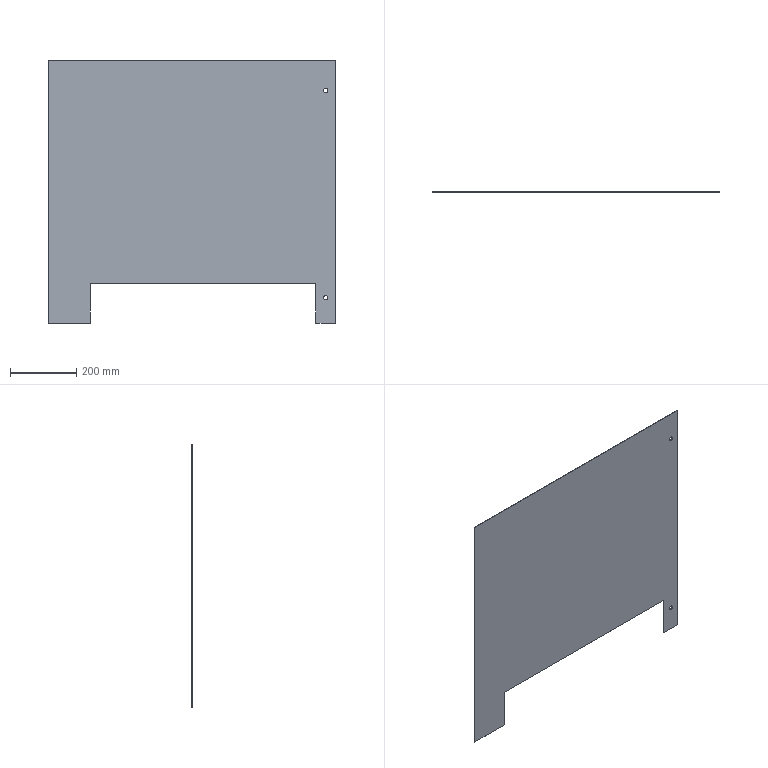Part | STEP file | E3-中转釜花纹Plate 4 | 1 solid | 14 faces | box 867 x 3 x 792 mm | volume 1814396 mm3 | plane 10 | cylinder 4 | commonest cylinder face diameters 13 x4
STEP:
#1=CARTESIAN_POINT('',(0.,0.,0.));
#2=DIRECTION('',(0.,0.,1.));
#3=DIRECTION('',(1.,0.,0.));
#4=AXIS2_PLACEMENT_3D('',#1,#2,#3);
#5=CARTESIAN_POINT('',(837.,0.,-49.5));
#6=VERTEX_POINT('',#5);
#7=CARTESIAN_POINT('',(837.,3.,-49.5));
#8=VERTEX_POINT('',#7);
#9=CARTESIAN_POINT('',(837.,11.,-49.5));
#10=DIRECTION('',(0.,1.,0.));
#11=VECTOR('',#10,1.);
#12=LINE('',#9,#11);
#13=CARTESIAN_POINT('',(837.,11.,-43.));
#14=DIRECTION('',(0.,1.,0.));
#15=DIRECTION('',(0.,0.,-1.));
#16=AXIS2_PLACEMENT_3D('',#13,#14,#15);
#17=CYLINDRICAL_SURFACE('',#16,6.5);
#18=CARTESIAN_POINT('',(6.283,0.));
#19=DIRECTION('',(0.,1.));
#20=VECTOR('',#19,1.);
#21=LINE('',#18,#20);
#22=(GEOMETRIC_REPRESENTATION_CONTEXT(2)PARAMETRIC_REPRESENTATION_CONTEXT()REPRESENTATION_CONTEXT('',''));
#23=DEFINITIONAL_REPRESENTATION('',(#21),#22);
#24=PCURVE('',#17,#23);
#25=CARTESIAN_POINT('',(837.,11.,-43.));
#26=DIRECTION('',(0.,1.,0.));
#27=DIRECTION('',(0.,0.,-1.));
#28=AXIS2_PLACEMENT_3D('',#25,#26,#27);
#29=CYLINDRICAL_SURFACE('',#28,6.5);
#30=CARTESIAN_POINT('',(0.,0.));
#31=DIRECTION('',(0.,1.));
#32=VECTOR('',#31,1.);
#33=LINE('',#30,#32);
#34=(GEOMETRIC_REPRESENTATION_CONTEXT(2)PARAMETRIC_REPRESENTATION_CONTEXT()REPRESENTATION_CONTEXT('',''));
#35=DEFINITIONAL_REPRESENTATION('',(#33),#34);
#36=PCURVE('',#29,#35);
#37=SURFACE_CURVE('',#12,(#24,#36),.PCURVE_S1.);
#38=EDGE_CURVE('',#6,#8,#37,.T.);
#39=ORIENTED_EDGE('',*,*,#38,.T.);
#40=CARTESIAN_POINT('',(837.,3.,-36.5));
#41=VERTEX_POINT('',#40);
#42=CARTESIAN_POINT('',(837.,3.,-43.));
#43=DIRECTION('',(0.,1.,0.));
#44=DIRECTION('',(0.,0.,1.));
#45=AXIS2_PLACEMENT_3D('',#42,#43,#44);
#46=CIRCLE('',#45,6.5);
#47=CARTESIAN_POINT('',(3.142,-8.));
#48=DIRECTION('',(1.,0.));
#49=VECTOR('',#48,1.);
#50=LINE('',#47,#49);
#51=(GEOMETRIC_REPRESENTATION_CONTEXT(2)PARAMETRIC_REPRESENTATION_CONTEXT()REPRESENTATION_CONTEXT('',''));
#52=DEFINITIONAL_REPRESENTATION('',(#50),#51);
#53=PCURVE('',#17,#52);
#54=CARTESIAN_POINT('',(0.,3.,0.));
#55=DIRECTION('',(0.,-1.,0.));
#56=DIRECTION('',(0.,0.,1.));
#57=AXIS2_PLACEMENT_3D('',#54,#55,#56);
#58=PLANE('',#57);
#59=CARTESIAN_POINT('',(-36.5,-837.));
#60=CARTESIAN_POINT('',(-36.5,-848.258));
#61=CARTESIAN_POINT('',(-46.25,-842.629));
#62=CARTESIAN_POINT('',(-56.,-837.));
#63=CARTESIAN_POINT('',(-46.25,-831.371));
#64=CARTESIAN_POINT('',(-36.5,-825.742));
#65=CARTESIAN_POINT('',(-36.5,-837.));
#66=(BOUNDED_CURVE()B_SPLINE_CURVE(2,(#59,#60,#61,#62,#63,#64,#65),.UNSPECIFIED.,.T.,.F.)B_SPLINE_CURVE_WITH_KNOTS((1,2,2,2,2,1),(-2.094,0.,2.094,4.189,6.283,8.378),.UNSPECIFIED.)CURVE()GEOMETRIC_REPRESENTATION_ITEM()RATIONAL_B_SPLINE_CURVE((1.,0.5,1.,0.5,1.,0.5,1.))REPRESENTATION_ITEM(''));
#67=(GEOMETRIC_REPRESENTATION_CONTEXT(2)PARAMETRIC_REPRESENTATION_CONTEXT()REPRESENTATION_CONTEXT('',''));
#68=DEFINITIONAL_REPRESENTATION('',(#66),#67);
#69=PCURVE('',#58,#68);
#70=SURFACE_CURVE('',#46,(#53,#69),.PCURVE_S1.);
#71=EDGE_CURVE('',#41,#8,#70,.T.);
#72=ORIENTED_EDGE('',*,*,#71,.F.);
#73=CARTESIAN_POINT('',(837.,0.,-36.5));
#74=VERTEX_POINT('',#73);
#75=CARTESIAN_POINT('',(837.,11.,-36.5));
#76=DIRECTION('',(0.,1.,0.));
#77=VECTOR('',#76,1.);
#78=LINE('',#75,#77);
#79=CARTESIAN_POINT('',(3.142,0.));
#80=DIRECTION('',(0.,1.));
#81=VECTOR('',#80,1.);
#82=LINE('',#79,#81);
#83=(GEOMETRIC_REPRESENTATION_CONTEXT(2)PARAMETRIC_REPRESENTATION_CONTEXT()REPRESENTATION_CONTEXT('',''));
#84=DEFINITIONAL_REPRESENTATION('',(#82),#83);
#85=PCURVE('',#17,#84);
#86=CARTESIAN_POINT('',(3.142,0.));
#87=DIRECTION('',(0.,1.));
#88=VECTOR('',#87,1.);
#89=LINE('',#86,#88);
#90=(GEOMETRIC_REPRESENTATION_CONTEXT(2)PARAMETRIC_REPRESENTATION_CONTEXT()REPRESENTATION_CONTEXT('',''));
#91=DEFINITIONAL_REPRESENTATION('',(#89),#90);
#92=PCURVE('',#29,#91);
#93=SURFACE_CURVE('',#78,(#85,#92),.PCURVE_S1.);
#94=EDGE_CURVE('',#74,#41,#93,.T.);
#95=ORIENTED_EDGE('',*,*,#94,.F.);
#96=CARTESIAN_POINT('',(837.,0.,-43.));
#97=DIRECTION('',(0.,1.,0.));
#98=DIRECTION('',(0.,0.,1.));
#99=AXIS2_PLACEMENT_3D('',#96,#97,#98);
#100=CIRCLE('',#99,6.5);
#101=CARTESIAN_POINT('',(3.142,-11.));
#102=DIRECTION('',(1.,0.));
#103=VECTOR('',#102,1.);
#104=LINE('',#101,#103);
#105=(GEOMETRIC_REPRESENTATION_CONTEXT(2)PARAMETRIC_REPRESENTATION_CONTEXT()REPRESENTATION_CONTEXT('',''));
#106=DEFINITIONAL_REPRESENTATION('',(#104),#105);
#107=PCURVE('',#17,#106);
#108=CARTESIAN_POINT('',(0.,0.,0.));
#109=DIRECTION('',(0.,-1.,0.));
#110=DIRECTION('',(0.,0.,1.));
#111=AXIS2_PLACEMENT_3D('',#108,#109,#110);
#112=PLANE('',#111);
#113=CARTESIAN_POINT('',(-36.5,-837.));
#114=CARTESIAN_POINT('',(-36.5,-848.258));
#115=CARTESIAN_POINT('',(-46.25,-842.629));
#116=CARTESIAN_POINT('',(-56.,-837.));
#117=CARTESIAN_POINT('',(-46.25,-831.371));
#118=CARTESIAN_POINT('',(-36.5,-825.742));
#119=CARTESIAN_POINT('',(-36.5,-837.));
#120=(BOUNDED_CURVE()B_SPLINE_CURVE(2,(#113,#114,#115,#116,#117,#118,#119),.UNSPECIFIED.,.T.,.F.)B_SPLINE_CURVE_WITH_KNOTS((1,2,2,2,2,1),(-2.094,0.,2.094,4.189,6.283,8.378),.UNSPECIFIED.)CURVE()GEOMETRIC_REPRESENTATION_ITEM()RATIONAL_B_SPLINE_CURVE((1.,0.5,1.,0.5,1.,0.5,1.))REPRESENTATION_ITEM(''));
#121=(GEOMETRIC_REPRESENTATION_CONTEXT(2)PARAMETRIC_REPRESENTATION_CONTEXT()REPRESENTATION_CONTEXT('',''));
#122=DEFINITIONAL_REPRESENTATION('',(#120),#121);
#123=PCURVE('',#112,#122);
#124=SURFACE_CURVE('',#100,(#107,#123),.PCURVE_S1.);
#125=EDGE_CURVE('',#74,#6,#124,.T.);
#126=ORIENTED_EDGE('',*,*,#125,.T.);
#127=EDGE_LOOP('',(#39,#72,#95,#126));
#128=FACE_BOUND('',#127,.F.);
#129=ADVANCED_FACE('',(#128),#17,.F.);
#130=CARTESIAN_POINT('',(837.,0.,575.5));
#131=VERTEX_POINT('',#130);
#132=CARTESIAN_POINT('',(837.,3.,575.5));
#133=VERTEX_POINT('',#132);
#134=CARTESIAN_POINT('',(837.,11.,575.5));
#135=DIRECTION('',(0.,1.,0.));
#136=VECTOR('',#135,1.);
#137=LINE('',#134,#136);
#138=CARTESIAN_POINT('',(837.,11.,582.));
#139=DIRECTION('',(0.,1.,0.));
#140=DIRECTION('',(0.,0.,-1.));
#141=AXIS2_PLACEMENT_3D('',#138,#139,#140);
#142=CYLINDRICAL_SURFACE('',#141,6.5);
#143=CARTESIAN_POINT('',(6.283,0.));
#144=DIRECTION('',(0.,1.));
#145=VECTOR('',#144,1.);
#146=LINE('',#143,#145);
#147=(GEOMETRIC_REPRESENTATION_CONTEXT(2)PARAMETRIC_REPRESENTATION_CONTEXT()REPRESENTATION_CONTEXT('',''));
#148=DEFINITIONAL_REPRESENTATION('',(#146),#147);
#149=PCURVE('',#142,#148);
#150=CARTESIAN_POINT('',(837.,11.,582.));
#151=DIRECTION('',(0.,1.,0.));
#152=DIRECTION('',(0.,0.,-1.));
#153=AXIS2_PLACEMENT_3D('',#150,#151,#152);
#154=CYLINDRICAL_SURFACE('',#153,6.5);
#155=CARTESIAN_POINT('',(0.,0.));
#156=DIRECTION('',(0.,1.));
#157=VECTOR('',#156,1.);
#158=LINE('',#155,#157);
#159=(GEOMETRIC_REPRESENTATION_CONTEXT(2)PARAMETRIC_REPRESENTATION_CONTEXT()REPRESENTATION_CONTEXT('',''));
#160=DEFINITIONAL_REPRESENTATION('',(#158),#159);
#161=PCURVE('',#154,#160);
#162=SURFACE_CURVE('',#137,(#149,#161),.PCURVE_S1.);
#163=EDGE_CURVE('',#131,#133,#162,.T.);
#164=ORIENTED_EDGE('',*,*,#163,.T.);
#165=CARTESIAN_POINT('',(837.,3.,588.5));
#166=VERTEX_POINT('',#165);
#167=CARTESIAN_POINT('',(837.,3.,582.));
#168=DIRECTION('',(0.,1.,0.));
#169=DIRECTION('',(0.,0.,1.));
#170=AXIS2_PLACEMENT_3D('',#167,#168,#169);
#171=CIRCLE('',#170,6.5);
#172=CARTESIAN_POINT('',(3.142,-8.));
#173=DIRECTION('',(1.,0.));
#174=VECTOR('',#173,1.);
#175=LINE('',#172,#174);
#176=(GEOMETRIC_REPRESENTATION_CONTEXT(2)PARAMETRIC_REPRESENTATION_CONTEXT()REPRESENTATION_CONTEXT('',''));
#177=DEFINITIONAL_REPRESENTATION('',(#175),#176);
#178=PCURVE('',#142,#177);
#179=CARTESIAN_POINT('',(588.5,-837.));
#180=CARTESIAN_POINT('',(588.5,-848.258));
#181=CARTESIAN_POINT('',(578.75,-842.629));
#182=CARTESIAN_POINT('',(569.,-837.));
#183=CARTESIAN_POINT('',(578.75,-831.371));
#184=CARTESIAN_POINT('',(588.5,-825.742));
#185=CARTESIAN_POINT('',(588.5,-837.));
#186=(BOUNDED_CURVE()B_SPLINE_CURVE(2,(#179,#180,#181,#182,#183,#184,#185),.UNSPECIFIED.,.T.,.F.)B_SPLINE_CURVE_WITH_KNOTS((1,2,2,2,2,1),(-2.094,0.,2.094,4.189,6.283,8.378),.UNSPECIFIED.)CURVE()GEOMETRIC_REPRESENTATION_ITEM()RATIONAL_B_SPLINE_CURVE((1.,0.5,1.,0.5,1.,0.5,1.))REPRESENTATION_ITEM(''));
#187=(GEOMETRIC_REPRESENTATION_CONTEXT(2)PARAMETRIC_REPRESENTATION_CONTEXT()REPRESENTATION_CONTEXT('',''));
#188=DEFINITIONAL_REPRESENTATION('',(#186),#187);
#189=PCURVE('',#58,#188);
#190=SURFACE_CURVE('',#171,(#178,#189),.PCURVE_S1.);
#191=EDGE_CURVE('',#166,#133,#190,.T.);
#192=ORIENTED_EDGE('',*,*,#191,.F.);
#193=CARTESIAN_POINT('',(837.,0.,588.5));
#194=VERTEX_POINT('',#193);
#195=CARTESIAN_POINT('',(837.,11.,588.5));
#196=DIRECTION('',(0.,1.,0.));
#197=VECTOR('',#196,1.);
#198=LINE('',#195,#197);
#199=CARTESIAN_POINT('',(3.142,0.));
#200=DIRECTION('',(0.,1.));
#201=VECTOR('',#200,1.);
#202=LINE('',#199,#201);
#203=(GEOMETRIC_REPRESENTATION_CONTEXT(2)PARAMETRIC_REPRESENTATION_CONTEXT()REPRESENTATION_CONTEXT('',''));
#204=DEFINITIONAL_REPRESENTATION('',(#202),#203);
#205=PCURVE('',#142,#204);
#206=CARTESIAN_POINT('',(3.142,0.));
#207=DIRECTION('',(0.,1.));
#208=VECTOR('',#207,1.);
#209=LINE('',#206,#208);
#210=(GEOMETRIC_REPRESENTATION_CONTEXT(2)PARAMETRIC_REPRESENTATION_CONTEXT()REPRESENTATION_CONTEXT('',''));
#211=DEFINITIONAL_REPRESENTATION('',(#209),#210);
#212=PCURVE('',#154,#211);
#213=SURFACE_CURVE('',#198,(#205,#212),.PCURVE_S1.);
#214=EDGE_CURVE('',#194,#166,#213,.T.);
#215=ORIENTED_EDGE('',*,*,#214,.F.);
#216=CARTESIAN_POINT('',(837.,0.,582.));
#217=DIRECTION('',(0.,1.,0.));
#218=DIRECTION('',(0.,0.,1.));
#219=AXIS2_PLACEMENT_3D('',#216,#217,#218);
#220=CIRCLE('',#219,6.5);
#221=CARTESIAN_POINT('',(3.142,-11.));
#222=DIRECTION('',(1.,0.));
#223=VECTOR('',#222,1.);
#224=LINE('',#221,#223);
#225=(GEOMETRIC_REPRESENTATION_CONTEXT(2)PARAMETRIC_REPRESENTATION_CONTEXT()REPRESENTATION_CONTEXT('',''));
#226=DEFINITIONAL_REPRESENTATION('',(#224),#225);
#227=PCURVE('',#142,#226);
#228=CARTESIAN_POINT('',(588.5,-837.));
#229=CARTESIAN_POINT('',(588.5,-848.258));
#230=CARTESIAN_POINT('',(578.75,-842.629));
#231=CARTESIAN_POINT('',(569.,-837.));
#232=CARTESIAN_POINT('',(578.75,-831.371));
#233=CARTESIAN_POINT('',(588.5,-825.742));
#234=CARTESIAN_POINT('',(588.5,-837.));
#235=(BOUNDED_CURVE()B_SPLINE_CURVE(2,(#228,#229,#230,#231,#232,#233,#234),.UNSPECIFIED.,.T.,.F.)B_SPLINE_CURVE_WITH_KNOTS((1,2,2,2,2,1),(-2.094,0.,2.094,4.189,6.283,8.378),.UNSPECIFIED.)CURVE()GEOMETRIC_REPRESENTATION_ITEM()RATIONAL_B_SPLINE_CURVE((1.,0.5,1.,0.5,1.,0.5,1.))REPRESENTATION_ITEM(''));
#236=(GEOMETRIC_REPRESENTATION_CONTEXT(2)PARAMETRIC_REPRESENTATION_CONTEXT()REPRESENTATION_CONTEXT('',''));
#237=DEFINITIONAL_REPRESENTATION('',(#235),#236);
#238=PCURVE('',#112,#237);
#239=SURFACE_CURVE('',#220,(#227,#238),.PCURVE_S1.);
#240=EDGE_CURVE('',#194,#131,#239,.T.);
#241=ORIENTED_EDGE('',*,*,#240,.T.);
#242=EDGE_LOOP('',(#164,#192,#215,#241));
#243=FACE_BOUND('',#242,.F.);
#244=ADVANCED_FACE('',(#243),#142,.F.);
#245=CARTESIAN_POINT('',(127.,0.,0.));
#246=VERTEX_POINT('',#245);
#247=CARTESIAN_POINT('',(807.,0.,0.));
#248=VERTEX_POINT('',#247);
#249=CARTESIAN_POINT('',(0.,0.,0.));
#250=DIRECTION('',(1.,0.,0.));
#251=VECTOR('',#250,1.);
#252=LINE('',#249,#251);
#253=CARTESIAN_POINT('',(0.,3.,0.));
#254=DIRECTION('',(0.,0.,1.));
#255=DIRECTION('',(-1.,0.,0.));
#256=AXIS2_PLACEMENT_3D('',#253,#254,#255);
#257=PLANE('',#256);
#258=CARTESIAN_POINT('',(0.,3.));
#259=DIRECTION('',(-1.,0.));
#260=VECTOR('',#259,1.);
#261=LINE('',#258,#260);
#262=(GEOMETRIC_REPRESENTATION_CONTEXT(2)PARAMETRIC_REPRESENTATION_CONTEXT()REPRESENTATION_CONTEXT('',''));
#263=DEFINITIONAL_REPRESENTATION('',(#261),#262);
#264=PCURVE('',#257,#263);
#265=CARTESIAN_POINT('',(0.,0.));
#266=DIRECTION('',(0.,-1.));
#267=VECTOR('',#266,1.);
#268=LINE('',#265,#267);
#269=(GEOMETRIC_REPRESENTATION_CONTEXT(2)PARAMETRIC_REPRESENTATION_CONTEXT()REPRESENTATION_CONTEXT('',''));
#270=DEFINITIONAL_REPRESENTATION('',(#268),#269);
#271=PCURVE('',#112,#270);
#272=SURFACE_CURVE('',#252,(#264,#271),.PCURVE_S1.);
#273=EDGE_CURVE('',#246,#248,#272,.T.);
#274=ORIENTED_EDGE('',*,*,#273,.F.);
#275=CARTESIAN_POINT('',(127.,3.,0.));
#276=VERTEX_POINT('',#275);
#277=CARTESIAN_POINT('',(127.,0.,0.));
#278=DIRECTION('',(0.,1.,0.));
#279=VECTOR('',#278,1.);
#280=LINE('',#277,#279);
#281=CARTESIAN_POINT('',(-127.,3.));
#282=DIRECTION('',(0.,-1.));
#283=VECTOR('',#282,1.);
#284=LINE('',#281,#283);
#285=(GEOMETRIC_REPRESENTATION_CONTEXT(2)PARAMETRIC_REPRESENTATION_CONTEXT()REPRESENTATION_CONTEXT('',''));
#286=DEFINITIONAL_REPRESENTATION('',(#284),#285);
#287=PCURVE('',#257,#286);
#288=CARTESIAN_POINT('',(127.,0.,0.));
#289=DIRECTION('',(1.,0.,0.));
#290=DIRECTION('',(0.,0.,1.));
#291=AXIS2_PLACEMENT_3D('',#288,#289,#290);
#292=PLANE('',#291);
#293=CARTESIAN_POINT('',(0.,0.));
#294=DIRECTION('',(0.,-1.));
#295=VECTOR('',#294,1.);
#296=LINE('',#293,#295);
#297=(GEOMETRIC_REPRESENTATION_CONTEXT(2)PARAMETRIC_REPRESENTATION_CONTEXT()REPRESENTATION_CONTEXT('',''));
#298=DEFINITIONAL_REPRESENTATION('',(#296),#297);
#299=PCURVE('',#292,#298);
#300=SURFACE_CURVE('',#280,(#287,#299),.PCURVE_S1.);
#301=EDGE_CURVE('',#246,#276,#300,.T.);
#302=ORIENTED_EDGE('',*,*,#301,.T.);
#303=CARTESIAN_POINT('',(807.,3.,0.));
#304=VERTEX_POINT('',#303);
#305=CARTESIAN_POINT('',(0.,3.,0.));
#306=DIRECTION('',(1.,0.,0.));
#307=VECTOR('',#306,1.);
#308=LINE('',#305,#307);
#309=CARTESIAN_POINT('',(0.,0.));
#310=DIRECTION('',(-1.,0.));
#311=VECTOR('',#310,1.);
#312=LINE('',#309,#311);
#313=(GEOMETRIC_REPRESENTATION_CONTEXT(2)PARAMETRIC_REPRESENTATION_CONTEXT()REPRESENTATION_CONTEXT('',''));
#314=DEFINITIONAL_REPRESENTATION('',(#312),#313);
#315=PCURVE('',#257,#314);
#316=CARTESIAN_POINT('',(0.,0.));
#317=DIRECTION('',(0.,-1.));
#318=VECTOR('',#317,1.);
#319=LINE('',#316,#318);
#320=(GEOMETRIC_REPRESENTATION_CONTEXT(2)PARAMETRIC_REPRESENTATION_CONTEXT()REPRESENTATION_CONTEXT('',''));
#321=DEFINITIONAL_REPRESENTATION('',(#319),#320);
#322=PCURVE('',#58,#321);
#323=SURFACE_CURVE('',#308,(#315,#322),.PCURVE_S1.);
#324=EDGE_CURVE('',#276,#304,#323,.T.);
#325=ORIENTED_EDGE('',*,*,#324,.T.);
#326=CARTESIAN_POINT('',(807.,0.,0.));
#327=DIRECTION('',(0.,1.,0.));
#328=VECTOR('',#327,1.);
#329=LINE('',#326,#328);
#330=CARTESIAN_POINT('',(-807.,3.));
#331=DIRECTION('',(0.,-1.));
#332=VECTOR('',#331,1.);
#333=LINE('',#330,#332);
#334=(GEOMETRIC_REPRESENTATION_CONTEXT(2)PARAMETRIC_REPRESENTATION_CONTEXT()REPRESENTATION_CONTEXT('',''));
#335=DEFINITIONAL_REPRESENTATION('',(#333),#334);
#336=PCURVE('',#257,#335);
#337=CARTESIAN_POINT('',(807.,0.,0.));
#338=DIRECTION('',(-1.,0.,0.));
#339=DIRECTION('',(0.,0.,-1.));
#340=AXIS2_PLACEMENT_3D('',#337,#338,#339);
#341=PLANE('',#340);
#342=CARTESIAN_POINT('',(0.,0.));
#343=DIRECTION('',(0.,-1.));
#344=VECTOR('',#343,1.);
#345=LINE('',#342,#344);
#346=(GEOMETRIC_REPRESENTATION_CONTEXT(2)PARAMETRIC_REPRESENTATION_CONTEXT()REPRESENTATION_CONTEXT('',''));
#347=DEFINITIONAL_REPRESENTATION('',(#345),#346);
#348=PCURVE('',#341,#347);
#349=SURFACE_CURVE('',#329,(#336,#348),.PCURVE_S1.);
#350=EDGE_CURVE('',#248,#304,#349,.T.);
#351=ORIENTED_EDGE('',*,*,#350,.F.);
#352=EDGE_LOOP('',(#274,#302,#325,#351));
#353=FACE_BOUND('',#352,.T.);
#354=ADVANCED_FACE('',(#353),#257,.F.);
#355=CARTESIAN_POINT('',(0.,0.,672.));
#356=VERTEX_POINT('',#355);
#357=CARTESIAN_POINT('',(0.,0.,-120.));
#358=VERTEX_POINT('',#357);
#359=CARTESIAN_POINT('',(0.,0.,0.));
#360=DIRECTION('',(0.,0.,-1.));
#361=VECTOR('',#360,1.);
#362=LINE('',#359,#361);
#363=CARTESIAN_POINT('',(0.,3.,0.));
#364=DIRECTION('',(1.,0.,0.));
#365=DIRECTION('',(0.,0.,1.));
#366=AXIS2_PLACEMENT_3D('',#363,#364,#365);
#367=PLANE('',#366);
#368=CARTESIAN_POINT('',(0.,3.));
#369=DIRECTION('',(-1.,0.));
#370=VECTOR('',#369,1.);
#371=LINE('',#368,#370);
#372=(GEOMETRIC_REPRESENTATION_CONTEXT(2)PARAMETRIC_REPRESENTATION_CONTEXT()REPRESENTATION_CONTEXT('',''));
#373=DEFINITIONAL_REPRESENTATION('',(#371),#372);
#374=PCURVE('',#367,#373);
#375=CARTESIAN_POINT('',(0.,0.));
#376=DIRECTION('',(-1.,0.));
#377=VECTOR('',#376,1.);
#378=LINE('',#375,#377);
#379=(GEOMETRIC_REPRESENTATION_CONTEXT(2)PARAMETRIC_REPRESENTATION_CONTEXT()REPRESENTATION_CONTEXT('',''));
#380=DEFINITIONAL_REPRESENTATION('',(#378),#379);
#381=PCURVE('',#112,#380);
#382=SURFACE_CURVE('',#362,(#374,#381),.PCURVE_S1.);
#383=EDGE_CURVE('',#356,#358,#382,.T.);
#384=ORIENTED_EDGE('',*,*,#383,.F.);
#385=CARTESIAN_POINT('',(0.,3.,672.));
#386=VERTEX_POINT('',#385);
#387=CARTESIAN_POINT('',(0.,3.,672.));
#388=DIRECTION('',(0.,-1.,0.));
#389=VECTOR('',#388,1.);
#390=LINE('',#387,#389);
#391=CARTESIAN_POINT('',(672.,0.));
#392=DIRECTION('',(0.,1.));
#393=VECTOR('',#392,1.);
#394=LINE('',#391,#393);
#395=(GEOMETRIC_REPRESENTATION_CONTEXT(2)PARAMETRIC_REPRESENTATION_CONTEXT()REPRESENTATION_CONTEXT('',''));
#396=DEFINITIONAL_REPRESENTATION('',(#394),#395);
#397=PCURVE('',#367,#396);
#398=CARTESIAN_POINT('',(0.,3.,672.));
#399=DIRECTION('',(0.,0.,-1.));
#400=DIRECTION('',(1.,0.,0.));
#401=AXIS2_PLACEMENT_3D('',#398,#399,#400);
#402=PLANE('',#401);
#403=CARTESIAN_POINT('',(0.,0.));
#404=DIRECTION('',(0.,1.));
#405=VECTOR('',#404,1.);
#406=LINE('',#403,#405);
#407=(GEOMETRIC_REPRESENTATION_CONTEXT(2)PARAMETRIC_REPRESENTATION_CONTEXT()REPRESENTATION_CONTEXT('',''));
#408=DEFINITIONAL_REPRESENTATION('',(#406),#407);
#409=PCURVE('',#402,#408);
#410=SURFACE_CURVE('',#390,(#397,#409),.PCURVE_S1.);
#411=EDGE_CURVE('',#386,#356,#410,.T.);
#412=ORIENTED_EDGE('',*,*,#411,.F.);
#413=CARTESIAN_POINT('',(0.,3.,-120.));
#414=VERTEX_POINT('',#413);
#415=CARTESIAN_POINT('',(0.,3.,0.));
#416=DIRECTION('',(0.,0.,-1.));
#417=VECTOR('',#416,1.);
#418=LINE('',#415,#417);
#419=CARTESIAN_POINT('',(0.,0.));
#420=DIRECTION('',(-1.,0.));
#421=VECTOR('',#420,1.);
#422=LINE('',#419,#421);
#423=(GEOMETRIC_REPRESENTATION_CONTEXT(2)PARAMETRIC_REPRESENTATION_CONTEXT()REPRESENTATION_CONTEXT('',''));
#424=DEFINITIONAL_REPRESENTATION('',(#422),#423);
#425=PCURVE('',#367,#424);
#426=CARTESIAN_POINT('',(0.,0.));
#427=DIRECTION('',(-1.,0.));
#428=VECTOR('',#427,1.);
#429=LINE('',#426,#428);
#430=(GEOMETRIC_REPRESENTATION_CONTEXT(2)PARAMETRIC_REPRESENTATION_CONTEXT()REPRESENTATION_CONTEXT('',''));
#431=DEFINITIONAL_REPRESENTATION('',(#429),#430);
#432=PCURVE('',#58,#431);
#433=SURFACE_CURVE('',#418,(#425,#432),.PCURVE_S1.);
#434=EDGE_CURVE('',#386,#414,#433,.T.);
#435=ORIENTED_EDGE('',*,*,#434,.T.);
#436=CARTESIAN_POINT('',(0.,0.,-120.));
#437=DIRECTION('',(0.,1.,0.));
#438=VECTOR('',#437,1.);
#439=LINE('',#436,#438);
#440=CARTESIAN_POINT('',(-120.,3.));
#441=DIRECTION('',(0.,-1.));
#442=VECTOR('',#441,1.);
#443=LINE('',#440,#442);
#444=(GEOMETRIC_REPRESENTATION_CONTEXT(2)PARAMETRIC_REPRESENTATION_CONTEXT()REPRESENTATION_CONTEXT('',''));
#445=DEFINITIONAL_REPRESENTATION('',(#443),#444);
#446=PCURVE('',#367,#445);
#447=CARTESIAN_POINT('',(0.,0.,-120.));
#448=DIRECTION('',(0.,0.,-1.));
#449=DIRECTION('',(1.,0.,0.));
#450=AXIS2_PLACEMENT_3D('',#447,#448,#449);
#451=PLANE('',#450);
#452=CARTESIAN_POINT('',(0.,0.));
#453=DIRECTION('',(0.,-1.));
#454=VECTOR('',#453,1.);
#455=LINE('',#452,#454);
#456=(GEOMETRIC_REPRESENTATION_CONTEXT(2)PARAMETRIC_REPRESENTATION_CONTEXT()REPRESENTATION_CONTEXT('',''));
#457=DEFINITIONAL_REPRESENTATION('',(#455),#456);
#458=PCURVE('',#451,#457);
#459=SURFACE_CURVE('',#439,(#446,#458),.PCURVE_S1.);
#460=EDGE_CURVE('',#358,#414,#459,.T.);
#461=ORIENTED_EDGE('',*,*,#460,.F.);
#462=EDGE_LOOP('',(#384,#412,#435,#461));
#463=FACE_BOUND('',#462,.T.);
#464=ADVANCED_FACE('',(#463),#367,.F.);
#465=CARTESIAN_POINT('',(867.,0.,-120.));
#466=VERTEX_POINT('',#465);
#467=CARTESIAN_POINT('',(867.,0.,672.));
#468=VERTEX_POINT('',#467);
#469=CARTESIAN_POINT('',(867.,0.,0.));
#470=DIRECTION('',(0.,0.,1.));
#471=VECTOR('',#470,1.);
#472=LINE('',#469,#471);
#473=CARTESIAN_POINT('',(867.,3.,0.));
#474=DIRECTION('',(-1.,0.,0.));
#475=DIRECTION('',(0.,0.,-1.));
#476=AXIS2_PLACEMENT_3D('',#473,#474,#475);
#477=PLANE('',#476);
#478=CARTESIAN_POINT('',(0.,3.));
#479=DIRECTION('',(-1.,0.));
#480=VECTOR('',#479,1.);
#481=LINE('',#478,#480);
#482=(GEOMETRIC_REPRESENTATION_CONTEXT(2)PARAMETRIC_REPRESENTATION_CONTEXT()REPRESENTATION_CONTEXT('',''));
#483=DEFINITIONAL_REPRESENTATION('',(#481),#482);
#484=PCURVE('',#477,#483);
#485=CARTESIAN_POINT('',(0.,-867.));
#486=DIRECTION('',(1.,0.));
#487=VECTOR('',#486,1.);
#488=LINE('',#485,#487);
#489=(GEOMETRIC_REPRESENTATION_CONTEXT(2)PARAMETRIC_REPRESENTATION_CONTEXT()REPRESENTATION_CONTEXT('',''));
#490=DEFINITIONAL_REPRESENTATION('',(#488),#489);
#491=PCURVE('',#112,#490);
#492=SURFACE_CURVE('',#472,(#484,#491),.PCURVE_S1.);
#493=EDGE_CURVE('',#466,#468,#492,.T.);
#494=ORIENTED_EDGE('',*,*,#493,.F.);
#495=CARTESIAN_POINT('',(867.,3.,-120.));
#496=VERTEX_POINT('',#495);
#497=CARTESIAN_POINT('',(867.,0.,-120.));
#498=DIRECTION('',(0.,1.,0.));
#499=VECTOR('',#498,1.);
#500=LINE('',#497,#499);
#501=CARTESIAN_POINT('',(120.,3.));
#502=DIRECTION('',(0.,-1.));
#503=VECTOR('',#502,1.);
#504=LINE('',#501,#503);
#505=(GEOMETRIC_REPRESENTATION_CONTEXT(2)PARAMETRIC_REPRESENTATION_CONTEXT()REPRESENTATION_CONTEXT('',''));
#506=DEFINITIONAL_REPRESENTATION('',(#504),#505);
#507=PCURVE('',#477,#506);
#508=CARTESIAN_POINT('',(867.,0.,-120.));
#509=DIRECTION('',(0.,0.,-1.));
#510=DIRECTION('',(1.,0.,0.));
#511=AXIS2_PLACEMENT_3D('',#508,#509,#510);
#512=PLANE('',#511);
#513=CARTESIAN_POINT('',(0.,0.));
#514=DIRECTION('',(0.,-1.));
#515=VECTOR('',#514,1.);
#516=LINE('',#513,#515);
#517=(GEOMETRIC_REPRESENTATION_CONTEXT(2)PARAMETRIC_REPRESENTATION_CONTEXT()REPRESENTATION_CONTEXT('',''));
#518=DEFINITIONAL_REPRESENTATION('',(#516),#517);
#519=PCURVE('',#512,#518);
#520=SURFACE_CURVE('',#500,(#507,#519),.PCURVE_S1.);
#521=EDGE_CURVE('',#466,#496,#520,.T.);
#522=ORIENTED_EDGE('',*,*,#521,.T.);
#523=CARTESIAN_POINT('',(867.,3.,672.));
#524=VERTEX_POINT('',#523);
#525=CARTESIAN_POINT('',(867.,3.,0.));
#526=DIRECTION('',(0.,0.,1.));
#527=VECTOR('',#526,1.);
#528=LINE('',#525,#527);
#529=CARTESIAN_POINT('',(0.,0.));
#530=DIRECTION('',(-1.,0.));
#531=VECTOR('',#530,1.);
#532=LINE('',#529,#531);
#533=(GEOMETRIC_REPRESENTATION_CONTEXT(2)PARAMETRIC_REPRESENTATION_CONTEXT()REPRESENTATION_CONTEXT('',''));
#534=DEFINITIONAL_REPRESENTATION('',(#532),#533);
#535=PCURVE('',#477,#534);
#536=CARTESIAN_POINT('',(0.,-867.));
#537=DIRECTION('',(1.,0.));
#538=VECTOR('',#537,1.);
#539=LINE('',#536,#538);
#540=(GEOMETRIC_REPRESENTATION_CONTEXT(2)PARAMETRIC_REPRESENTATION_CONTEXT()REPRESENTATION_CONTEXT('',''));
#541=DEFINITIONAL_REPRESENTATION('',(#539),#540);
#542=PCURVE('',#58,#541);
#543=SURFACE_CURVE('',#528,(#535,#542),.PCURVE_S1.);
#544=EDGE_CURVE('',#496,#524,#543,.T.);
#545=ORIENTED_EDGE('',*,*,#544,.T.);
#546=CARTESIAN_POINT('',(867.,3.,672.));
#547=DIRECTION('',(0.,-1.,0.));
#548=VECTOR('',#547,1.);
#549=LINE('',#546,#548);
#550=CARTESIAN_POINT('',(-672.,0.));
#551=DIRECTION('',(0.,1.));
#552=VECTOR('',#551,1.);
#553=LINE('',#550,#552);
#554=(GEOMETRIC_REPRESENTATION_CONTEXT(2)PARAMETRIC_REPRESENTATION_CONTEXT()REPRESENTATION_CONTEXT('',''));
#555=DEFINITIONAL_REPRESENTATION('',(#553),#554);
#556=PCURVE('',#477,#555);
#557=CARTESIAN_POINT('',(867.,0.));
#558=DIRECTION('',(0.,1.));
#559=VECTOR('',#558,1.);
#560=LINE('',#557,#559);
#561=(GEOMETRIC_REPRESENTATION_CONTEXT(2)PARAMETRIC_REPRESENTATION_CONTEXT()REPRESENTATION_CONTEXT('',''));
#562=DEFINITIONAL_REPRESENTATION('',(#560),#561);
#563=PCURVE('',#402,#562);
#564=SURFACE_CURVE('',#549,(#556,#563),.PCURVE_S1.);
#565=EDGE_CURVE('',#524,#468,#564,.T.);
#566=ORIENTED_EDGE('',*,*,#565,.T.);
#567=EDGE_LOOP('',(#494,#522,#545,#566));
#568=FACE_BOUND('',#567,.T.);
#569=ADVANCED_FACE('',(#568),#477,.F.);
#570=CARTESIAN_POINT('',(0.,0.,672.));
#571=DIRECTION('',(-1.,0.,0.));
#572=VECTOR('',#571,1.);
#573=LINE('',#570,#572);
#574=CARTESIAN_POINT('',(0.,3.));
#575=DIRECTION('',(-1.,0.));
#576=VECTOR('',#575,1.);
#577=LINE('',#574,#576);
#578=(GEOMETRIC_REPRESENTATION_CONTEXT(2)PARAMETRIC_REPRESENTATION_CONTEXT()REPRESENTATION_CONTEXT('',''));
#579=DEFINITIONAL_REPRESENTATION('',(#577),#578);
#580=PCURVE('',#402,#579);
#581=CARTESIAN_POINT('',(672.,0.));
#582=DIRECTION('',(0.,1.));
#583=VECTOR('',#582,1.);
#584=LINE('',#581,#583);
#585=(GEOMETRIC_REPRESENTATION_CONTEXT(2)PARAMETRIC_REPRESENTATION_CONTEXT()REPRESENTATION_CONTEXT('',''));
#586=DEFINITIONAL_REPRESENTATION('',(#584),#585);
#587=PCURVE('',#112,#586);
#588=SURFACE_CURVE('',#573,(#580,#587),.PCURVE_S1.);
#589=EDGE_CURVE('',#468,#356,#588,.T.);
#590=ORIENTED_EDGE('',*,*,#589,.F.);
#591=ORIENTED_EDGE('',*,*,#565,.F.);
#592=CARTESIAN_POINT('',(0.,3.,672.));
#593=DIRECTION('',(-1.,0.,0.));
#594=VECTOR('',#593,1.);
#595=LINE('',#592,#594);
#596=CARTESIAN_POINT('',(0.,0.));
#597=DIRECTION('',(-1.,0.));
#598=VECTOR('',#597,1.);
#599=LINE('',#596,#598);
#600=(GEOMETRIC_REPRESENTATION_CONTEXT(2)PARAMETRIC_REPRESENTATION_CONTEXT()REPRESENTATION_CONTEXT('',''));
#601=DEFINITIONAL_REPRESENTATION('',(#599),#600);
#602=PCURVE('',#402,#601);
#603=CARTESIAN_POINT('',(672.,0.));
#604=DIRECTION('',(0.,1.));
#605=VECTOR('',#604,1.);
#606=LINE('',#603,#605);
#607=(GEOMETRIC_REPRESENTATION_CONTEXT(2)PARAMETRIC_REPRESENTATION_CONTEXT()REPRESENTATION_CONTEXT('',''));
#608=DEFINITIONAL_REPRESENTATION('',(#606),#607);
#609=PCURVE('',#58,#608);
#610=SURFACE_CURVE('',#595,(#602,#609),.PCURVE_S1.);
#611=EDGE_CURVE('',#524,#386,#610,.T.);
#612=ORIENTED_EDGE('',*,*,#611,.T.);
#613=ORIENTED_EDGE('',*,*,#411,.T.);
#614=EDGE_LOOP('',(#590,#591,#612,#613));
#615=FACE_BOUND('',#614,.T.);
#616=ADVANCED_FACE('',(#615),#402,.F.);
#617=CARTESIAN_POINT('',(837.,3.,-43.));
#618=DIRECTION('',(0.,1.,0.));
#619=DIRECTION('',(0.,0.,1.));
#620=AXIS2_PLACEMENT_3D('',#617,#618,#619);
#621=CIRCLE('',#620,6.5);
#622=CARTESIAN_POINT('',(-36.5,-837.));
#623=CARTESIAN_POINT('',(-36.5,-848.258));
#624=CARTESIAN_POINT('',(-46.25,-842.629));
#625=CARTESIAN_POINT('',(-56.,-837.));
#626=CARTESIAN_POINT('',(-46.25,-831.371));
#627=CARTESIAN_POINT('',(-36.5,-825.742));
#628=CARTESIAN_POINT('',(-36.5,-837.));
#629=(BOUNDED_CURVE()B_SPLINE_CURVE(2,(#622,#623,#624,#625,#626,#627,#628),.UNSPECIFIED.,.T.,.F.)B_SPLINE_CURVE_WITH_KNOTS((1,2,2,2,2,1),(-2.094,0.,2.094,4.189,6.283,8.378),.UNSPECIFIED.)CURVE()GEOMETRIC_REPRESENTATION_ITEM()RATIONAL_B_SPLINE_CURVE((1.,0.5,1.,0.5,1.,0.5,1.))REPRESENTATION_ITEM(''));
#630=(GEOMETRIC_REPRESENTATION_CONTEXT(2)PARAMETRIC_REPRESENTATION_CONTEXT()REPRESENTATION_CONTEXT('',''));
#631=DEFINITIONAL_REPRESENTATION('',(#629),#630);
#632=PCURVE('',#58,#631);
#633=CARTESIAN_POINT('',(-3.142,-8.));
#634=DIRECTION('',(1.,0.));
#635=VECTOR('',#634,1.);
#636=LINE('',#633,#635);
#637=(GEOMETRIC_REPRESENTATION_CONTEXT(2)PARAMETRIC_REPRESENTATION_CONTEXT()REPRESENTATION_CONTEXT('',''));
#638=DEFINITIONAL_REPRESENTATION('',(#636),#637);
#639=PCURVE('',#29,#638);
#640=SURFACE_CURVE('',#621,(#632,#639),.PCURVE_S1.);
#641=EDGE_CURVE('',#8,#41,#640,.T.);
#642=ORIENTED_EDGE('',*,*,#641,.F.);
#643=ORIENTED_EDGE('',*,*,#71,.F.);
#644=EDGE_LOOP('',(#642,#643));
#645=FACE_BOUND('',#644,.T.);
#646=CARTESIAN_POINT('',(837.,3.,582.));
#647=DIRECTION('',(0.,1.,0.));
#648=DIRECTION('',(0.,0.,1.));
#649=AXIS2_PLACEMENT_3D('',#646,#647,#648);
#650=CIRCLE('',#649,6.5);
#651=CARTESIAN_POINT('',(588.5,-837.));
#652=CARTESIAN_POINT('',(588.5,-848.258));
#653=CARTESIAN_POINT('',(578.75,-842.629));
#654=CARTESIAN_POINT('',(569.,-837.));
#655=CARTESIAN_POINT('',(578.75,-831.371));
#656=CARTESIAN_POINT('',(588.5,-825.742));
#657=CARTESIAN_POINT('',(588.5,-837.));
#658=(BOUNDED_CURVE()B_SPLINE_CURVE(2,(#651,#652,#653,#654,#655,#656,#657),.UNSPECIFIED.,.T.,.F.)B_SPLINE_CURVE_WITH_KNOTS((1,2,2,2,2,1),(-2.094,0.,2.094,4.189,6.283,8.378),.UNSPECIFIED.)CURVE()GEOMETRIC_REPRESENTATION_ITEM()RATIONAL_B_SPLINE_CURVE((1.,0.5,1.,0.5,1.,0.5,1.))REPRESENTATION_ITEM(''));
#659=(GEOMETRIC_REPRESENTATION_CONTEXT(2)PARAMETRIC_REPRESENTATION_CONTEXT()REPRESENTATION_CONTEXT('',''));
#660=DEFINITIONAL_REPRESENTATION('',(#658),#659);
#661=PCURVE('',#58,#660);
#662=CARTESIAN_POINT('',(-3.142,-8.));
#663=DIRECTION('',(1.,0.));
#664=VECTOR('',#663,1.);
#665=LINE('',#662,#664);
#666=(GEOMETRIC_REPRESENTATION_CONTEXT(2)PARAMETRIC_REPRESENTATION_CONTEXT()REPRESENTATION_CONTEXT('',''));
#667=DEFINITIONAL_REPRESENTATION('',(#665),#666);
#668=PCURVE('',#154,#667);
#669=SURFACE_CURVE('',#650,(#661,#668),.PCURVE_S1.);
#670=EDGE_CURVE('',#133,#166,#669,.T.);
#671=ORIENTED_EDGE('',*,*,#670,.F.);
#672=ORIENTED_EDGE('',*,*,#191,.F.);
#673=EDGE_LOOP('',(#671,#672));
#674=FACE_BOUND('',#673,.T.);
#675=ORIENTED_EDGE('',*,*,#434,.F.);
#676=ORIENTED_EDGE('',*,*,#611,.F.);
#677=ORIENTED_EDGE('',*,*,#544,.F.);
#678=CARTESIAN_POINT('',(807.,3.,-120.));
#679=VERTEX_POINT('',#678);
#680=CARTESIAN_POINT('',(867.,3.,-120.));
#681=DIRECTION('',(1.,0.,0.));
#682=VECTOR('',#681,1.);
#683=LINE('',#680,#682);
#684=CARTESIAN_POINT('',(-120.,-867.));
#685=DIRECTION('',(0.,-1.));
#686=VECTOR('',#685,1.);
#687=LINE('',#684,#686);
#688=(GEOMETRIC_REPRESENTATION_CONTEXT(2)PARAMETRIC_REPRESENTATION_CONTEXT()REPRESENTATION_CONTEXT('',''));
#689=DEFINITIONAL_REPRESENTATION('',(#687),#688);
#690=PCURVE('',#58,#689);
#691=CARTESIAN_POINT('',(0.,-3.));
#692=DIRECTION('',(1.,0.));
#693=VECTOR('',#692,1.);
#694=LINE('',#691,#693);
#695=(GEOMETRIC_REPRESENTATION_CONTEXT(2)PARAMETRIC_REPRESENTATION_CONTEXT()REPRESENTATION_CONTEXT('',''));
#696=DEFINITIONAL_REPRESENTATION('',(#694),#695);
#697=PCURVE('',#512,#696);
#698=SURFACE_CURVE('',#683,(#690,#697),.PCURVE_S1.);
#699=EDGE_CURVE('',#679,#496,#698,.T.);
#700=ORIENTED_EDGE('',*,*,#699,.F.);
#701=CARTESIAN_POINT('',(807.,3.,0.));
#702=DIRECTION('',(0.,0.,-1.));
#703=VECTOR('',#702,1.);
#704=LINE('',#701,#703);
#705=CARTESIAN_POINT('',(0.,-807.));
#706=DIRECTION('',(-1.,0.));
#707=VECTOR('',#706,1.);
#708=LINE('',#705,#707);
#709=(GEOMETRIC_REPRESENTATION_CONTEXT(2)PARAMETRIC_REPRESENTATION_CONTEXT()REPRESENTATION_CONTEXT('',''));
#710=DEFINITIONAL_REPRESENTATION('',(#708),#709);
#711=PCURVE('',#58,#710);
#712=CARTESIAN_POINT('',(0.,-3.));
#713=DIRECTION('',(1.,0.));
#714=VECTOR('',#713,1.);
#715=LINE('',#712,#714);
#716=(GEOMETRIC_REPRESENTATION_CONTEXT(2)PARAMETRIC_REPRESENTATION_CONTEXT()REPRESENTATION_CONTEXT('',''));
#717=DEFINITIONAL_REPRESENTATION('',(#715),#716);
#718=PCURVE('',#341,#717);
#719=SURFACE_CURVE('',#704,(#711,#718),.PCURVE_S1.);
#720=EDGE_CURVE('',#304,#679,#719,.T.);
#721=ORIENTED_EDGE('',*,*,#720,.F.);
#722=ORIENTED_EDGE('',*,*,#324,.F.);
#723=CARTESIAN_POINT('',(127.,3.,-120.));
#724=VERTEX_POINT('',#723);
#725=CARTESIAN_POINT('',(127.,3.,0.));
#726=DIRECTION('',(0.,0.,1.));
#727=VECTOR('',#726,1.);
#728=LINE('',#725,#727);
#729=CARTESIAN_POINT('',(0.,-127.));
#730=DIRECTION('',(1.,0.));
#731=VECTOR('',#730,1.);
#732=LINE('',#729,#731);
#733=(GEOMETRIC_REPRESENTATION_CONTEXT(2)PARAMETRIC_REPRESENTATION_CONTEXT()REPRESENTATION_CONTEXT('',''));
#734=DEFINITIONAL_REPRESENTATION('',(#732),#733);
#735=PCURVE('',#58,#734);
#736=CARTESIAN_POINT('',(0.,-3.));
#737=DIRECTION('',(1.,0.));
#738=VECTOR('',#737,1.);
#739=LINE('',#736,#738);
#740=(GEOMETRIC_REPRESENTATION_CONTEXT(2)PARAMETRIC_REPRESENTATION_CONTEXT()REPRESENTATION_CONTEXT('',''));
#741=DEFINITIONAL_REPRESENTATION('',(#739),#740);
#742=PCURVE('',#292,#741);
#743=SURFACE_CURVE('',#728,(#735,#742),.PCURVE_S1.);
#744=EDGE_CURVE('',#724,#276,#743,.T.);
#745=ORIENTED_EDGE('',*,*,#744,.F.);
#746=CARTESIAN_POINT('',(0.,3.,-120.));
#747=DIRECTION('',(1.,0.,0.));
#748=VECTOR('',#747,1.);
#749=LINE('',#746,#748);
#750=CARTESIAN_POINT('',(-120.,0.));
#751=DIRECTION('',(0.,-1.));
#752=VECTOR('',#751,1.);
#753=LINE('',#750,#752);
#754=(GEOMETRIC_REPRESENTATION_CONTEXT(2)PARAMETRIC_REPRESENTATION_CONTEXT()REPRESENTATION_CONTEXT('',''));
#755=DEFINITIONAL_REPRESENTATION('',(#753),#754);
#756=PCURVE('',#58,#755);
#757=CARTESIAN_POINT('',(0.,-3.));
#758=DIRECTION('',(1.,0.));
#759=VECTOR('',#758,1.);
#760=LINE('',#757,#759);
#761=(GEOMETRIC_REPRESENTATION_CONTEXT(2)PARAMETRIC_REPRESENTATION_CONTEXT()REPRESENTATION_CONTEXT('',''));
#762=DEFINITIONAL_REPRESENTATION('',(#760),#761);
#763=PCURVE('',#451,#762);
#764=SURFACE_CURVE('',#749,(#756,#763),.PCURVE_S1.);
#765=EDGE_CURVE('',#414,#724,#764,.T.);
#766=ORIENTED_EDGE('',*,*,#765,.F.);
#767=EDGE_LOOP('',(#675,#676,#677,#700,#721,#722,#745,#766));
#768=FACE_BOUND('',#767,.T.);
#769=ADVANCED_FACE('',(#645,#674,#768),#58,.F.);
#770=CARTESIAN_POINT('',(837.,0.,-43.));
#771=DIRECTION('',(0.,1.,0.));
#772=DIRECTION('',(0.,0.,1.));
#773=AXIS2_PLACEMENT_3D('',#770,#771,#772);
#774=CIRCLE('',#773,6.5);
#775=CARTESIAN_POINT('',(-36.5,-837.));
#776=CARTESIAN_POINT('',(-36.5,-848.258));
#777=CARTESIAN_POINT('',(-46.25,-842.629));
#778=CARTESIAN_POINT('',(-56.,-837.));
#779=CARTESIAN_POINT('',(-46.25,-831.371));
#780=CARTESIAN_POINT('',(-36.5,-825.742));
#781=CARTESIAN_POINT('',(-36.5,-837.));
#782=(BOUNDED_CURVE()B_SPLINE_CURVE(2,(#775,#776,#777,#778,#779,#780,#781),.UNSPECIFIED.,.T.,.F.)B_SPLINE_CURVE_WITH_KNOTS((1,2,2,2,2,1),(-2.094,0.,2.094,4.189,6.283,8.378),.UNSPECIFIED.)CURVE()GEOMETRIC_REPRESENTATION_ITEM()RATIONAL_B_SPLINE_CURVE((1.,0.5,1.,0.5,1.,0.5,1.))REPRESENTATION_ITEM(''));
#783=(GEOMETRIC_REPRESENTATION_CONTEXT(2)PARAMETRIC_REPRESENTATION_CONTEXT()REPRESENTATION_CONTEXT('',''));
#784=DEFINITIONAL_REPRESENTATION('',(#782),#783);
#785=PCURVE('',#112,#784);
#786=CARTESIAN_POINT('',(-3.142,-11.));
#787=DIRECTION('',(1.,0.));
#788=VECTOR('',#787,1.);
#789=LINE('',#786,#788);
#790=(GEOMETRIC_REPRESENTATION_CONTEXT(2)PARAMETRIC_REPRESENTATION_CONTEXT()REPRESENTATION_CONTEXT('',''));
#791=DEFINITIONAL_REPRESENTATION('',(#789),#790);
#792=PCURVE('',#29,#791);
#793=SURFACE_CURVE('',#774,(#785,#792),.PCURVE_S1.);
#794=EDGE_CURVE('',#6,#74,#793,.T.);
#795=ORIENTED_EDGE('',*,*,#794,.T.);
#796=ORIENTED_EDGE('',*,*,#125,.T.);
#797=EDGE_LOOP('',(#795,#796));
#798=FACE_BOUND('',#797,.T.);
#799=CARTESIAN_POINT('',(837.,0.,582.));
#800=DIRECTION('',(0.,1.,0.));
#801=DIRECTION('',(0.,0.,1.));
#802=AXIS2_PLACEMENT_3D('',#799,#800,#801);
#803=CIRCLE('',#802,6.5);
#804=CARTESIAN_POINT('',(588.5,-837.));
#805=CARTESIAN_POINT('',(588.5,-848.258));
#806=CARTESIAN_POINT('',(578.75,-842.629));
#807=CARTESIAN_POINT('',(569.,-837.));
#808=CARTESIAN_POINT('',(578.75,-831.371));
#809=CARTESIAN_POINT('',(588.5,-825.742));
#810=CARTESIAN_POINT('',(588.5,-837.));
#811=(BOUNDED_CURVE()B_SPLINE_CURVE(2,(#804,#805,#806,#807,#808,#809,#810),.UNSPECIFIED.,.T.,.F.)B_SPLINE_CURVE_WITH_KNOTS((1,2,2,2,2,1),(-2.094,0.,2.094,4.189,6.283,8.378),.UNSPECIFIED.)CURVE()GEOMETRIC_REPRESENTATION_ITEM()RATIONAL_B_SPLINE_CURVE((1.,0.5,1.,0.5,1.,0.5,1.))REPRESENTATION_ITEM(''));
#812=(GEOMETRIC_REPRESENTATION_CONTEXT(2)PARAMETRIC_REPRESENTATION_CONTEXT()REPRESENTATION_CONTEXT('',''));
#813=DEFINITIONAL_REPRESENTATION('',(#811),#812);
#814=PCURVE('',#112,#813);
#815=CARTESIAN_POINT('',(-3.142,-11.));
#816=DIRECTION('',(1.,0.));
#817=VECTOR('',#816,1.);
#818=LINE('',#815,#817);
#819=(GEOMETRIC_REPRESENTATION_CONTEXT(2)PARAMETRIC_REPRESENTATION_CONTEXT()REPRESENTATION_CONTEXT('',''));
#820=DEFINITIONAL_REPRESENTATION('',(#818),#819);
#821=PCURVE('',#154,#820);
#822=SURFACE_CURVE('',#803,(#814,#821),.PCURVE_S1.);
#823=EDGE_CURVE('',#131,#194,#822,.T.);
#824=ORIENTED_EDGE('',*,*,#823,.T.);
#825=ORIENTED_EDGE('',*,*,#240,.T.);
#826=EDGE_LOOP('',(#824,#825));
#827=FACE_BOUND('',#826,.T.);
#828=ORIENTED_EDGE('',*,*,#383,.T.);
#829=CARTESIAN_POINT('',(127.,0.,-120.));
#830=VERTEX_POINT('',#829);
#831=CARTESIAN_POINT('',(0.,0.,-120.));
#832=DIRECTION('',(1.,0.,0.));
#833=VECTOR('',#832,1.);
#834=LINE('',#831,#833);
#835=CARTESIAN_POINT('',(-120.,0.));
#836=DIRECTION('',(0.,-1.));
#837=VECTOR('',#836,1.);
#838=LINE('',#835,#837);
#839=(GEOMETRIC_REPRESENTATION_CONTEXT(2)PARAMETRIC_REPRESENTATION_CONTEXT()REPRESENTATION_CONTEXT('',''));
#840=DEFINITIONAL_REPRESENTATION('',(#838),#839);
#841=PCURVE('',#112,#840);
#842=CARTESIAN_POINT('',(0.,0.));
#843=DIRECTION('',(1.,0.));
#844=VECTOR('',#843,1.);
#845=LINE('',#842,#844);
#846=(GEOMETRIC_REPRESENTATION_CONTEXT(2)PARAMETRIC_REPRESENTATION_CONTEXT()REPRESENTATION_CONTEXT('',''));
#847=DEFINITIONAL_REPRESENTATION('',(#845),#846);
#848=PCURVE('',#451,#847);
#849=SURFACE_CURVE('',#834,(#841,#848),.PCURVE_S1.);
#850=EDGE_CURVE('',#358,#830,#849,.T.);
#851=ORIENTED_EDGE('',*,*,#850,.T.);
#852=CARTESIAN_POINT('',(127.,0.,0.));
#853=DIRECTION('',(0.,0.,1.));
#854=VECTOR('',#853,1.);
#855=LINE('',#852,#854);
#856=CARTESIAN_POINT('',(0.,-127.));
#857=DIRECTION('',(1.,0.));
#858=VECTOR('',#857,1.);
#859=LINE('',#856,#858);
#860=(GEOMETRIC_REPRESENTATION_CONTEXT(2)PARAMETRIC_REPRESENTATION_CONTEXT()REPRESENTATION_CONTEXT('',''));
#861=DEFINITIONAL_REPRESENTATION('',(#859),#860);
#862=PCURVE('',#112,#861);
#863=CARTESIAN_POINT('',(0.,0.));
#864=DIRECTION('',(1.,0.));
#865=VECTOR('',#864,1.);
#866=LINE('',#863,#865);
#867=(GEOMETRIC_REPRESENTATION_CONTEXT(2)PARAMETRIC_REPRESENTATION_CONTEXT()REPRESENTATION_CONTEXT('',''));
#868=DEFINITIONAL_REPRESENTATION('',(#866),#867);
#869=PCURVE('',#292,#868);
#870=SURFACE_CURVE('',#855,(#862,#869),.PCURVE_S1.);
#871=EDGE_CURVE('',#830,#246,#870,.T.);
#872=ORIENTED_EDGE('',*,*,#871,.T.);
#873=ORIENTED_EDGE('',*,*,#273,.T.);
#874=CARTESIAN_POINT('',(807.,0.,-120.));
#875=VERTEX_POINT('',#874);
#876=CARTESIAN_POINT('',(807.,0.,0.));
#877=DIRECTION('',(0.,0.,-1.));
#878=VECTOR('',#877,1.);
#879=LINE('',#876,#878);
#880=CARTESIAN_POINT('',(0.,-807.));
#881=DIRECTION('',(-1.,0.));
#882=VECTOR('',#881,1.);
#883=LINE('',#880,#882);
#884=(GEOMETRIC_REPRESENTATION_CONTEXT(2)PARAMETRIC_REPRESENTATION_CONTEXT()REPRESENTATION_CONTEXT('',''));
#885=DEFINITIONAL_REPRESENTATION('',(#883),#884);
#886=PCURVE('',#112,#885);
#887=CARTESIAN_POINT('',(0.,0.));
#888=DIRECTION('',(1.,0.));
#889=VECTOR('',#888,1.);
#890=LINE('',#887,#889);
#891=(GEOMETRIC_REPRESENTATION_CONTEXT(2)PARAMETRIC_REPRESENTATION_CONTEXT()REPRESENTATION_CONTEXT('',''));
#892=DEFINITIONAL_REPRESENTATION('',(#890),#891);
#893=PCURVE('',#341,#892);
#894=SURFACE_CURVE('',#879,(#886,#893),.PCURVE_S1.);
#895=EDGE_CURVE('',#248,#875,#894,.T.);
#896=ORIENTED_EDGE('',*,*,#895,.T.);
#897=CARTESIAN_POINT('',(867.,0.,-120.));
#898=DIRECTION('',(1.,0.,0.));
#899=VECTOR('',#898,1.);
#900=LINE('',#897,#899);
#901=CARTESIAN_POINT('',(-120.,-867.));
#902=DIRECTION('',(0.,-1.));
#903=VECTOR('',#902,1.);
#904=LINE('',#901,#903);
#905=(GEOMETRIC_REPRESENTATION_CONTEXT(2)PARAMETRIC_REPRESENTATION_CONTEXT()REPRESENTATION_CONTEXT('',''));
#906=DEFINITIONAL_REPRESENTATION('',(#904),#905);
#907=PCURVE('',#112,#906);
#908=CARTESIAN_POINT('',(0.,0.));
#909=DIRECTION('',(1.,0.));
#910=VECTOR('',#909,1.);
#911=LINE('',#908,#910);
#912=(GEOMETRIC_REPRESENTATION_CONTEXT(2)PARAMETRIC_REPRESENTATION_CONTEXT()REPRESENTATION_CONTEXT('',''));
#913=DEFINITIONAL_REPRESENTATION('',(#911),#912);
#914=PCURVE('',#512,#913);
#915=SURFACE_CURVE('',#900,(#907,#914),.PCURVE_S1.);
#916=EDGE_CURVE('',#875,#466,#915,.T.);
#917=ORIENTED_EDGE('',*,*,#916,.T.);
#918=ORIENTED_EDGE('',*,*,#493,.T.);
#919=ORIENTED_EDGE('',*,*,#589,.T.);
#920=EDGE_LOOP('',(#828,#851,#872,#873,#896,#917,#918,#919));
#921=FACE_BOUND('',#920,.T.);
#922=ADVANCED_FACE('',(#798,#827,#921),#112,.T.);
#923=ORIENTED_EDGE('',*,*,#744,.T.);
#924=ORIENTED_EDGE('',*,*,#301,.F.);
#925=ORIENTED_EDGE('',*,*,#871,.F.);
#926=CARTESIAN_POINT('',(127.,0.,-120.));
#927=DIRECTION('',(0.,1.,0.));
#928=VECTOR('',#927,1.);
#929=LINE('',#926,#928);
#930=CARTESIAN_POINT('',(-120.,0.));
#931=DIRECTION('',(0.,-1.));
#932=VECTOR('',#931,1.);
#933=LINE('',#930,#932);
#934=(GEOMETRIC_REPRESENTATION_CONTEXT(2)PARAMETRIC_REPRESENTATION_CONTEXT()REPRESENTATION_CONTEXT('',''));
#935=DEFINITIONAL_REPRESENTATION('',(#933),#934);
#936=PCURVE('',#292,#935);
#937=CARTESIAN_POINT('',(127.,0.));
#938=DIRECTION('',(0.,-1.));
#939=VECTOR('',#938,1.);
#940=LINE('',#937,#939);
#941=(GEOMETRIC_REPRESENTATION_CONTEXT(2)PARAMETRIC_REPRESENTATION_CONTEXT()REPRESENTATION_CONTEXT('',''));
#942=DEFINITIONAL_REPRESENTATION('',(#940),#941);
#943=PCURVE('',#451,#942);
#944=SURFACE_CURVE('',#929,(#936,#943),.PCURVE_S1.);
#945=EDGE_CURVE('',#830,#724,#944,.T.);
#946=ORIENTED_EDGE('',*,*,#945,.T.);
#947=EDGE_LOOP('',(#923,#924,#925,#946));
#948=FACE_BOUND('',#947,.T.);
#949=ADVANCED_FACE('',(#948),#292,.T.);
#950=ORIENTED_EDGE('',*,*,#765,.T.);
#951=ORIENTED_EDGE('',*,*,#945,.F.);
#952=ORIENTED_EDGE('',*,*,#850,.F.);
#953=ORIENTED_EDGE('',*,*,#460,.T.);
#954=EDGE_LOOP('',(#950,#951,#952,#953));
#955=FACE_BOUND('',#954,.T.);
#956=ADVANCED_FACE('',(#955),#451,.T.);
#957=ORIENTED_EDGE('',*,*,#699,.T.);
#958=ORIENTED_EDGE('',*,*,#521,.F.);
#959=ORIENTED_EDGE('',*,*,#916,.F.);
#960=CARTESIAN_POINT('',(807.,0.,-120.));
#961=DIRECTION('',(0.,1.,0.));
#962=VECTOR('',#961,1.);
#963=LINE('',#960,#962);
#964=CARTESIAN_POINT('',(-60.,0.));
#965=DIRECTION('',(0.,-1.));
#966=VECTOR('',#965,1.);
#967=LINE('',#964,#966);
#968=(GEOMETRIC_REPRESENTATION_CONTEXT(2)PARAMETRIC_REPRESENTATION_CONTEXT()REPRESENTATION_CONTEXT('',''));
#969=DEFINITIONAL_REPRESENTATION('',(#967),#968);
#970=PCURVE('',#512,#969);
#971=CARTESIAN_POINT('',(120.,0.));
#972=DIRECTION('',(0.,-1.));
#973=VECTOR('',#972,1.);
#974=LINE('',#971,#973);
#975=(GEOMETRIC_REPRESENTATION_CONTEXT(2)PARAMETRIC_REPRESENTATION_CONTEXT()REPRESENTATION_CONTEXT('',''));
#976=DEFINITIONAL_REPRESENTATION('',(#974),#975);
#977=PCURVE('',#341,#976);
#978=SURFACE_CURVE('',#963,(#970,#977),.PCURVE_S1.);
#979=EDGE_CURVE('',#875,#679,#978,.T.);
#980=ORIENTED_EDGE('',*,*,#979,.T.);
#981=EDGE_LOOP('',(#957,#958,#959,#980));
#982=FACE_BOUND('',#981,.T.);
#983=ADVANCED_FACE('',(#982),#512,.T.);
#984=ORIENTED_EDGE('',*,*,#720,.T.);
#985=ORIENTED_EDGE('',*,*,#979,.F.);
#986=ORIENTED_EDGE('',*,*,#895,.F.);
#987=ORIENTED_EDGE('',*,*,#350,.T.);
#988=EDGE_LOOP('',(#984,#985,#986,#987));
#989=FACE_BOUND('',#988,.T.);
#990=ADVANCED_FACE('',(#989),#341,.T.);
#991=ORIENTED_EDGE('',*,*,#670,.F.);
#992=ORIENTED_EDGE('',*,*,#163,.F.);
#993=ORIENTED_EDGE('',*,*,#823,.T.);
#994=ORIENTED_EDGE('',*,*,#214,.T.);
#995=EDGE_LOOP('',(#991,#992,#993,#994));
#996=FACE_BOUND('',#995,.F.);
#997=ADVANCED_FACE('',(#996),#154,.F.);
#998=ORIENTED_EDGE('',*,*,#641,.F.);
#999=ORIENTED_EDGE('',*,*,#38,.F.);
#1000=ORIENTED_EDGE('',*,*,#794,.T.);
#1001=ORIENTED_EDGE('',*,*,#94,.T.);
#1002=EDGE_LOOP('',(#998,#999,#1000,#1001));
#1003=FACE_BOUND('',#1002,.F.);
#1004=ADVANCED_FACE('',(#1003),#29,.F.);
#1005=CLOSED_SHELL('',(#129,#244,#354,#464,#569,#616,#769,#922,#949,#956,#983,#990,#997,#1004));
#1006=MANIFOLD_SOLID_BREP('',#1005);
#1007=(LENGTH_UNIT()NAMED_UNIT(*)SI_UNIT(.MILLI.,.METRE.));
#1008=UNCERTAINTY_MEASURE_WITH_UNIT(LENGTH_MEASURE(0.0000001),#1007,'','');
#1009=(NAMED_UNIT(*)PLANE_ANGLE_UNIT()SI_UNIT($,.RADIAN.));
#1010=(NAMED_UNIT(*)SI_UNIT($,.STERADIAN.)SOLID_ANGLE_UNIT());
#1011=(GEOMETRIC_REPRESENTATION_CONTEXT(3)GLOBAL_UNCERTAINTY_ASSIGNED_CONTEXT((#1008))GLOBAL_UNIT_ASSIGNED_CONTEXT((#1007,#1009,#1010))REPRESENTATION_CONTEXT('',''));
#1012=ADVANCED_BREP_SHAPE_REPRESENTATION('',(#4,#1006),#1011);